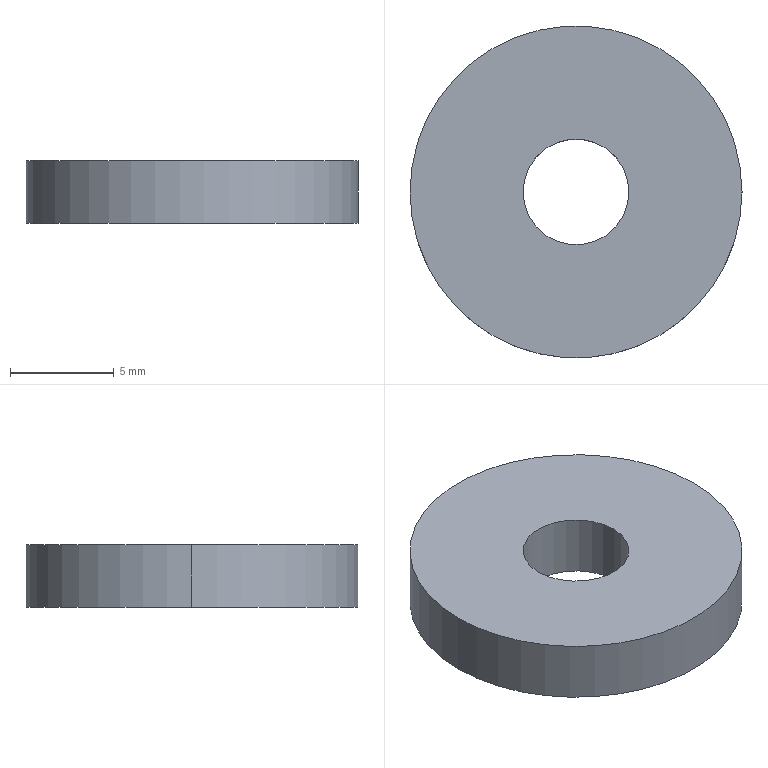Part | NX | features BREP 1 | 1 solid | 6 faces | box 16 x 16 x 3 mm | volume 541.901 mm3 | cylinder 4 | plane 2 | commonest cylinder face diameters 5.1 x2 16 x2
STEP:
#1=CARTESIAN_POINT('',(-2.55,0.,3.));
#2=VERTEX_POINT('',#1);
#3=CARTESIAN_POINT('',(2.55,0.,3.));
#4=VERTEX_POINT('',#3);
#5=CARTESIAN_POINT('',(0.,0.,3.));
#6=DIRECTION('',(0.,0.,1.));
#7=DIRECTION('',(1.,0.,0.));
#8=AXIS2_PLACEMENT_3D('',#5,#6,#7);
#9=CIRCLE('',#8,2.55);
#10=EDGE_CURVE('',#2,#4,#9,.T.);
#11=ORIENTED_EDGE('',*,*,#10,.T.);
#12=CARTESIAN_POINT('',(2.55,0.,0.));
#13=VERTEX_POINT('',#12);
#14=CARTESIAN_POINT('',(2.55,0.,3.));
#15=DIRECTION('',(0.,0.,-1.));
#16=VECTOR('',#15,1000.);
#17=LINE('',#14,#16);
#18=EDGE_CURVE('',#4,#13,#17,.T.);
#19=ORIENTED_EDGE('',*,*,#18,.T.);
#20=CARTESIAN_POINT('',(-2.55,0.,0.));
#21=VERTEX_POINT('',#20);
#22=CARTESIAN_POINT('',(0.,0.,0.));
#23=DIRECTION('',(0.,0.,1.));
#24=DIRECTION('',(1.,0.,0.));
#25=AXIS2_PLACEMENT_3D('',#22,#23,#24);
#26=CIRCLE('',#25,2.55);
#27=EDGE_CURVE('',#21,#13,#26,.T.);
#28=ORIENTED_EDGE('',*,*,#27,.F.);
#29=CARTESIAN_POINT('',(-2.55,0.,3.));
#30=DIRECTION('',(0.,0.,-1.));
#31=VECTOR('',#30,1000.);
#32=LINE('',#29,#31);
#33=EDGE_CURVE('',#2,#21,#32,.T.);
#34=ORIENTED_EDGE('',*,*,#33,.F.);
#35=EDGE_LOOP('',(#11,#19,#28,#34));
#36=FACE_BOUND('',#35,.T.);
#37=CARTESIAN_POINT('',(0.,0.,3.));
#38=DIRECTION('',(0.,0.,-1.));
#39=DIRECTION('',(-1.,0.,0.));
#40=AXIS2_PLACEMENT_3D('',#37,#38,#39);
#41=CYLINDRICAL_SURFACE('',#40,2.55);
#42=ADVANCED_FACE('',(#36),#41,.F.);
#43=CARTESIAN_POINT('',(8.,0.,3.));
#44=VERTEX_POINT('',#43);
#45=CARTESIAN_POINT('',(-8.,0.,3.));
#46=VERTEX_POINT('',#45);
#47=CARTESIAN_POINT('',(0.,0.,3.));
#48=DIRECTION('',(0.,0.,1.));
#49=DIRECTION('',(1.,0.,0.));
#50=AXIS2_PLACEMENT_3D('',#47,#48,#49);
#51=CIRCLE('',#50,8.);
#52=EDGE_CURVE('',#44,#46,#51,.T.);
#53=ORIENTED_EDGE('',*,*,#52,.F.);
#54=CARTESIAN_POINT('',(8.,0.,0.));
#55=VERTEX_POINT('',#54);
#56=CARTESIAN_POINT('',(8.,0.,3.));
#57=DIRECTION('',(0.,0.,-1.));
#58=VECTOR('',#57,1000.);
#59=LINE('',#56,#58);
#60=EDGE_CURVE('',#44,#55,#59,.T.);
#61=ORIENTED_EDGE('',*,*,#60,.T.);
#62=CARTESIAN_POINT('',(-8.,0.,0.));
#63=VERTEX_POINT('',#62);
#64=CARTESIAN_POINT('',(0.,0.,0.));
#65=DIRECTION('',(0.,0.,1.));
#66=DIRECTION('',(1.,0.,0.));
#67=AXIS2_PLACEMENT_3D('',#64,#65,#66);
#68=CIRCLE('',#67,8.);
#69=EDGE_CURVE('',#55,#63,#68,.T.);
#70=ORIENTED_EDGE('',*,*,#69,.T.);
#71=CARTESIAN_POINT('',(-8.,0.,3.));
#72=DIRECTION('',(0.,0.,-1.));
#73=VECTOR('',#72,1000.);
#74=LINE('',#71,#73);
#75=EDGE_CURVE('',#46,#63,#74,.T.);
#76=ORIENTED_EDGE('',*,*,#75,.F.);
#77=EDGE_LOOP('',(#53,#61,#70,#76));
#78=FACE_BOUND('',#77,.T.);
#79=CARTESIAN_POINT('',(0.,0.,3.));
#80=DIRECTION('',(0.,0.,-1.));
#81=DIRECTION('',(-1.,0.,0.));
#82=AXIS2_PLACEMENT_3D('',#79,#80,#81);
#83=CYLINDRICAL_SURFACE('',#82,8.);
#84=ADVANCED_FACE('',(#78),#83,.T.);
#85=CARTESIAN_POINT('',(0.,0.,3.));
#86=DIRECTION('',(0.,0.,1.));
#87=DIRECTION('',(1.,0.,0.));
#88=AXIS2_PLACEMENT_3D('',#85,#86,#87);
#89=CIRCLE('',#88,8.);
#90=EDGE_CURVE('',#46,#44,#89,.T.);
#91=ORIENTED_EDGE('',*,*,#90,.T.);
#92=ORIENTED_EDGE('',*,*,#52,.T.);
#93=EDGE_LOOP('',(#91,#92));
#94=FACE_BOUND('',#93,.T.);
#95=ORIENTED_EDGE('',*,*,#10,.F.);
#96=CARTESIAN_POINT('',(0.,0.,3.));
#97=DIRECTION('',(0.,0.,1.));
#98=DIRECTION('',(1.,0.,0.));
#99=AXIS2_PLACEMENT_3D('',#96,#97,#98);
#100=CIRCLE('',#99,2.55);
#101=EDGE_CURVE('',#4,#2,#100,.T.);
#102=ORIENTED_EDGE('',*,*,#101,.F.);
#103=EDGE_LOOP('',(#95,#102));
#104=FACE_BOUND('',#103,.T.);
#105=CARTESIAN_POINT('',(0.,0.,3.));
#106=DIRECTION('',(0.,0.,1.));
#107=DIRECTION('',(1.,0.,0.));
#108=AXIS2_PLACEMENT_3D('',#105,#106,#107);
#109=PLANE('',#108);
#110=ADVANCED_FACE('',(#94,#104),#109,.T.);
#111=CARTESIAN_POINT('',(0.,0.,0.));
#112=DIRECTION('',(0.,0.,1.));
#113=DIRECTION('',(1.,0.,0.));
#114=AXIS2_PLACEMENT_3D('',#111,#112,#113);
#115=CIRCLE('',#114,8.);
#116=EDGE_CURVE('',#63,#55,#115,.T.);
#117=ORIENTED_EDGE('',*,*,#116,.F.);
#118=ORIENTED_EDGE('',*,*,#69,.F.);
#119=EDGE_LOOP('',(#117,#118));
#120=FACE_BOUND('',#119,.T.);
#121=ORIENTED_EDGE('',*,*,#27,.T.);
#122=CARTESIAN_POINT('',(0.,0.,0.));
#123=DIRECTION('',(0.,0.,1.));
#124=DIRECTION('',(1.,0.,0.));
#125=AXIS2_PLACEMENT_3D('',#122,#123,#124);
#126=CIRCLE('',#125,2.55);
#127=EDGE_CURVE('',#13,#21,#126,.T.);
#128=ORIENTED_EDGE('',*,*,#127,.T.);
#129=EDGE_LOOP('',(#121,#128));
#130=FACE_BOUND('',#129,.T.);
#131=CARTESIAN_POINT('',(0.,0.,0.));
#132=DIRECTION('',(0.,0.,1.));
#133=DIRECTION('',(1.,0.,0.));
#134=AXIS2_PLACEMENT_3D('',#131,#132,#133);
#135=PLANE('',#134);
#136=ADVANCED_FACE('',(#120,#130),#135,.F.);
#137=ORIENTED_EDGE('',*,*,#60,.F.);
#138=ORIENTED_EDGE('',*,*,#90,.F.);
#139=ORIENTED_EDGE('',*,*,#75,.T.);
#140=ORIENTED_EDGE('',*,*,#116,.T.);
#141=EDGE_LOOP('',(#137,#138,#139,#140));
#142=FACE_BOUND('',#141,.T.);
#143=CARTESIAN_POINT('',(0.,0.,3.));
#144=DIRECTION('',(0.,0.,-1.));
#145=DIRECTION('',(-1.,0.,0.));
#146=AXIS2_PLACEMENT_3D('',#143,#144,#145);
#147=CYLINDRICAL_SURFACE('',#146,8.);
#148=ADVANCED_FACE('',(#142),#147,.T.);
#149=ORIENTED_EDGE('',*,*,#18,.F.);
#150=ORIENTED_EDGE('',*,*,#101,.T.);
#151=ORIENTED_EDGE('',*,*,#33,.T.);
#152=ORIENTED_EDGE('',*,*,#127,.F.);
#153=EDGE_LOOP('',(#149,#150,#151,#152));
#154=FACE_BOUND('',#153,.T.);
#155=CARTESIAN_POINT('',(0.,0.,3.));
#156=DIRECTION('',(0.,0.,-1.));
#157=DIRECTION('',(-1.,0.,0.));
#158=AXIS2_PLACEMENT_3D('',#155,#156,#157);
#159=CYLINDRICAL_SURFACE('',#158,2.55);
#160=ADVANCED_FACE('',(#154),#159,.F.);
#161=CLOSED_SHELL('',(#42,#84,#110,#136,#148,#160));
#162=MANIFOLD_SOLID_BREP('',#161);
#163=(LENGTH_UNIT()NAMED_UNIT(*)SI_UNIT(.MILLI.,.METRE.));
#164=UNCERTAINTY_MEASURE_WITH_UNIT(LENGTH_MEASURE(0.00001),#163,'','');
#165=(NAMED_UNIT(*)PLANE_ANGLE_UNIT()SI_UNIT($,.RADIAN.));
#166=(NAMED_UNIT(*)SI_UNIT($,.STERADIAN.)SOLID_ANGLE_UNIT());
#167=(GEOMETRIC_REPRESENTATION_CONTEXT(3)GLOBAL_UNCERTAINTY_ASSIGNED_CONTEXT((#164))GLOBAL_UNIT_ASSIGNED_CONTEXT((#163,#165,#166))REPRESENTATION_CONTEXT('',''));
#168=ADVANCED_BREP_SHAPE_REPRESENTATION('',(#162),#167);